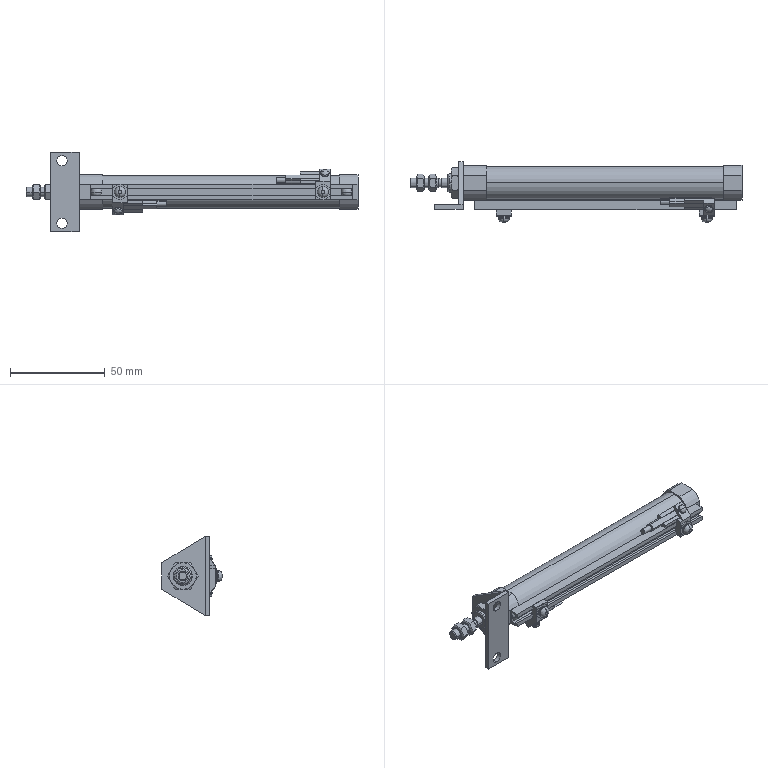Part | SolidWorks | 12 solids | 304 faces | box 175 x 31.65 x 42 mm | volume 27316 mm3 | plane 152 | cylinder 84 | cone 44 | torus 20 | sphere 4 | commonest cylinder face diameters 4.134 x10 3 x8 20 x8 4 x6 5 x6 0.6 x4